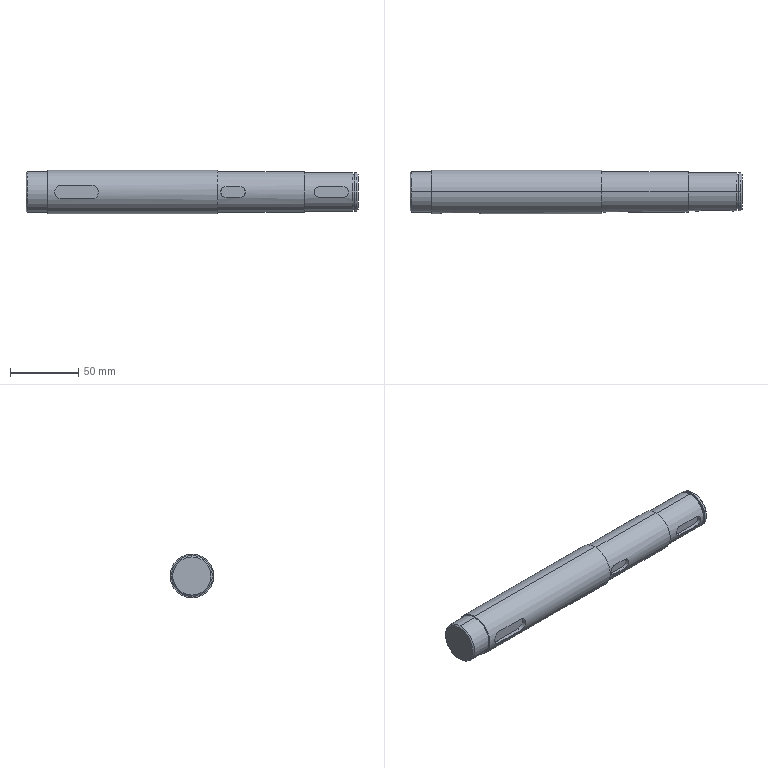Part | SolidWorks | features BaseBody 1 | 1 solid | 38 faces | box 243 x 32 x 32 mm | volume 178150 mm3 | cylinder 18 | plane 16 | cone 4 | commonest cylinder face diameters 8 x4 28 x4 30 x4 10 x2 25 x2 32 x2
STEP:
#1=CARTESIAN_POINT('',(16.,0.,-16.));
#2=VERTEX_POINT('',#1);
#3=CARTESIAN_POINT('',(16.,0.,16.));
#4=VERTEX_POINT('',#3);
#5=CARTESIAN_POINT('',(16.,0.,0.));
#6=DIRECTION('',(1.,0.,0.));
#7=DIRECTION('',(0.,0.,-1.));
#8=AXIS2_PLACEMENT_3D('',#5,#6,#7);
#9=CIRCLE('',#8,16.);
#10=EDGE_CURVE('',#2,#4,#9,.T.);
#11=ORIENTED_EDGE('',*,*,#10,.T.);
#12=CARTESIAN_POINT('',(140.5,0.,16.));
#13=VERTEX_POINT('',#12);
#14=CARTESIAN_POINT('',(78.25,0.,16.));
#15=DIRECTION('',(1.,0.,0.));
#16=VECTOR('',#15,1000.);
#17=LINE('',#14,#16);
#18=EDGE_CURVE('',#4,#13,#17,.T.);
#19=ORIENTED_EDGE('',*,*,#18,.T.);
#20=CARTESIAN_POINT('',(140.5,0.,-16.));
#21=VERTEX_POINT('',#20);
#22=CARTESIAN_POINT('',(140.5,0.,0.));
#23=DIRECTION('',(-1.,0.,0.));
#24=DIRECTION('',(0.,0.,-1.));
#25=AXIS2_PLACEMENT_3D('',#22,#23,#24);
#26=CIRCLE('',#25,16.);
#27=EDGE_CURVE('',#13,#21,#26,.T.);
#28=ORIENTED_EDGE('',*,*,#27,.T.);
#29=CARTESIAN_POINT('',(78.25,0.,-16.));
#30=DIRECTION('',(1.,0.,0.));
#31=VECTOR('',#30,1000.);
#32=LINE('',#29,#31);
#33=EDGE_CURVE('',#2,#21,#32,.T.);
#34=ORIENTED_EDGE('',*,*,#33,.F.);
#35=EDGE_LOOP('',(#11,#19,#28,#34));
#36=FACE_OUTER_BOUND('',#35,.T.);
#37=CARTESIAN_POINT('',(78.25,0.,0.));
#38=DIRECTION('',(1.,0.,0.));
#39=DIRECTION('',(0.,0.,-1.));
#40=AXIS2_PLACEMENT_3D('',#37,#38,#39);
#41=CYLINDRICAL_SURFACE('',#40,16.);
#42=ADVANCED_FACE('',(#36),#41,.T.);
#43=CARTESIAN_POINT('',(1.,0.,-15.));
#44=VERTEX_POINT('',#43);
#45=CARTESIAN_POINT('',(1.,0.,15.));
#46=VERTEX_POINT('',#45);
#47=CARTESIAN_POINT('',(1.,0.,0.));
#48=DIRECTION('',(1.,0.,0.));
#49=DIRECTION('',(0.,0.,-1.));
#50=AXIS2_PLACEMENT_3D('',#47,#48,#49);
#51=CIRCLE('',#50,15.);
#52=EDGE_CURVE('',#44,#46,#51,.T.);
#53=ORIENTED_EDGE('',*,*,#52,.T.);
#54=CARTESIAN_POINT('',(16.,0.,15.));
#55=VERTEX_POINT('',#54);
#56=CARTESIAN_POINT('',(8.,0.,15.));
#57=DIRECTION('',(1.,0.,0.));
#58=VECTOR('',#57,1000.);
#59=LINE('',#56,#58);
#60=EDGE_CURVE('',#46,#55,#59,.T.);
#61=ORIENTED_EDGE('',*,*,#60,.T.);
#62=CARTESIAN_POINT('',(16.,0.,-15.));
#63=VERTEX_POINT('',#62);
#64=CARTESIAN_POINT('',(16.,0.,0.));
#65=DIRECTION('',(1.,0.,0.));
#66=DIRECTION('',(0.,0.,-1.));
#67=AXIS2_PLACEMENT_3D('',#64,#65,#66);
#68=CIRCLE('',#67,15.);
#69=EDGE_CURVE('',#63,#55,#68,.T.);
#70=ORIENTED_EDGE('',*,*,#69,.F.);
#71=CARTESIAN_POINT('',(8.,0.,-15.));
#72=DIRECTION('',(1.,0.,0.));
#73=VECTOR('',#72,1000.);
#74=LINE('',#71,#73);
#75=EDGE_CURVE('',#44,#63,#74,.T.);
#76=ORIENTED_EDGE('',*,*,#75,.F.);
#77=EDGE_LOOP('',(#53,#61,#70,#76));
#78=FACE_OUTER_BOUND('',#77,.T.);
#79=CARTESIAN_POINT('',(8.,0.,0.));
#80=DIRECTION('',(1.,0.,0.));
#81=DIRECTION('',(0.,0.,-1.));
#82=AXIS2_PLACEMENT_3D('',#79,#80,#81);
#83=CYLINDRICAL_SURFACE('',#82,15.);
#84=ADVANCED_FACE('',(#78),#83,.T.);
#85=CARTESIAN_POINT('',(140.5,0.,15.));
#86=VERTEX_POINT('',#85);
#87=CARTESIAN_POINT('',(140.5,0.,-15.));
#88=VERTEX_POINT('',#87);
#89=CARTESIAN_POINT('',(140.5,0.,0.));
#90=DIRECTION('',(-1.,0.,0.));
#91=DIRECTION('',(0.,0.,-1.));
#92=AXIS2_PLACEMENT_3D('',#89,#90,#91);
#93=CIRCLE('',#92,15.);
#94=EDGE_CURVE('',#86,#88,#93,.T.);
#95=ORIENTED_EDGE('',*,*,#94,.F.);
#96=CARTESIAN_POINT('',(203.5,0.,15.));
#97=VERTEX_POINT('',#96);
#98=CARTESIAN_POINT('',(172.,0.,15.));
#99=DIRECTION('',(1.,0.,0.));
#100=VECTOR('',#99,1000.);
#101=LINE('',#98,#100);
#102=EDGE_CURVE('',#86,#97,#101,.T.);
#103=ORIENTED_EDGE('',*,*,#102,.T.);
#104=CARTESIAN_POINT('',(203.5,0.,-15.));
#105=VERTEX_POINT('',#104);
#106=CARTESIAN_POINT('',(203.5,0.,0.));
#107=DIRECTION('',(-1.,0.,0.));
#108=DIRECTION('',(0.,0.,-1.));
#109=AXIS2_PLACEMENT_3D('',#106,#107,#108);
#110=CIRCLE('',#109,15.);
#111=EDGE_CURVE('',#97,#105,#110,.T.);
#112=ORIENTED_EDGE('',*,*,#111,.T.);
#113=CARTESIAN_POINT('',(172.,0.,-15.));
#114=DIRECTION('',(1.,0.,0.));
#115=VECTOR('',#114,1000.);
#116=LINE('',#113,#115);
#117=EDGE_CURVE('',#88,#105,#116,.T.);
#118=ORIENTED_EDGE('',*,*,#117,.F.);
#119=EDGE_LOOP('',(#95,#103,#112,#118));
#120=FACE_OUTER_BOUND('',#119,.T.);
#121=CARTESIAN_POINT('',(172.,0.,0.));
#122=DIRECTION('',(1.,0.,0.));
#123=DIRECTION('',(0.,0.,-1.));
#124=AXIS2_PLACEMENT_3D('',#121,#122,#123);
#125=CYLINDRICAL_SURFACE('',#124,15.);
#126=ADVANCED_FACE('',(#120),#125,.T.);
#127=CARTESIAN_POINT('',(0.,0.,-14.));
#128=VERTEX_POINT('',#127);
#129=CARTESIAN_POINT('',(0.,0.,14.));
#130=VERTEX_POINT('',#129);
#131=CARTESIAN_POINT('',(0.,0.,0.));
#132=DIRECTION('',(1.,0.,0.));
#133=DIRECTION('',(0.,0.,-1.));
#134=AXIS2_PLACEMENT_3D('',#131,#132,#133);
#135=CIRCLE('',#134,14.);
#136=EDGE_CURVE('',#128,#130,#135,.T.);
#137=ORIENTED_EDGE('',*,*,#136,.T.);
#138=CARTESIAN_POINT('',(1.,0.,15.));
#139=DIRECTION('',(0.7071,0.,0.7071));
#140=VECTOR('',#139,1000.);
#141=LINE('',#138,#140);
#142=EDGE_CURVE('',#130,#46,#141,.T.);
#143=ORIENTED_EDGE('',*,*,#142,.T.);
#144=ORIENTED_EDGE('',*,*,#52,.F.);
#145=CARTESIAN_POINT('',(1.,0.,-15.));
#146=DIRECTION('',(0.7071,0.,-0.7071));
#147=VECTOR('',#146,1000.);
#148=LINE('',#145,#147);
#149=EDGE_CURVE('',#128,#44,#148,.T.);
#150=ORIENTED_EDGE('',*,*,#149,.F.);
#151=EDGE_LOOP('',(#137,#143,#144,#150));
#152=FACE_OUTER_BOUND('',#151,.T.);
#153=CARTESIAN_POINT('',(1.,0.,0.));
#154=DIRECTION('',(1.,0.,0.));
#155=DIRECTION('',(0.,0.,-1.));
#156=AXIS2_PLACEMENT_3D('',#153,#154,#155);
#157=CONICAL_SURFACE('',#156,15.,0.7854);
#158=ADVANCED_FACE('',(#152),#157,.T.);
#159=CARTESIAN_POINT('',(203.5,0.,14.));
#160=VERTEX_POINT('',#159);
#161=CARTESIAN_POINT('',(203.5,0.,-14.));
#162=VERTEX_POINT('',#161);
#163=CARTESIAN_POINT('',(203.5,0.,0.));
#164=DIRECTION('',(-1.,0.,0.));
#165=DIRECTION('',(0.,0.,-1.));
#166=AXIS2_PLACEMENT_3D('',#163,#164,#165);
#167=CIRCLE('',#166,14.);
#168=EDGE_CURVE('',#160,#162,#167,.T.);
#169=ORIENTED_EDGE('',*,*,#168,.F.);
#170=CARTESIAN_POINT('',(239.,0.,14.));
#171=VERTEX_POINT('',#170);
#172=CARTESIAN_POINT('',(221.25,0.,14.));
#173=DIRECTION('',(1.,0.,0.));
#174=VECTOR('',#173,1000.);
#175=LINE('',#172,#174);
#176=EDGE_CURVE('',#160,#171,#175,.T.);
#177=ORIENTED_EDGE('',*,*,#176,.T.);
#178=CARTESIAN_POINT('',(239.,0.,-14.));
#179=VERTEX_POINT('',#178);
#180=CARTESIAN_POINT('',(239.,0.,0.));
#181=DIRECTION('',(-1.,0.,0.));
#182=DIRECTION('',(0.,0.,-1.));
#183=AXIS2_PLACEMENT_3D('',#180,#181,#182);
#184=CIRCLE('',#183,14.);
#185=EDGE_CURVE('',#171,#179,#184,.T.);
#186=ORIENTED_EDGE('',*,*,#185,.T.);
#187=CARTESIAN_POINT('',(221.25,0.,-14.));
#188=DIRECTION('',(1.,0.,0.));
#189=VECTOR('',#188,1000.);
#190=LINE('',#187,#189);
#191=EDGE_CURVE('',#162,#179,#190,.T.);
#192=ORIENTED_EDGE('',*,*,#191,.F.);
#193=EDGE_LOOP('',(#169,#177,#186,#192));
#194=FACE_OUTER_BOUND('',#193,.T.);
#195=CARTESIAN_POINT('',(221.25,0.,0.));
#196=DIRECTION('',(1.,0.,0.));
#197=DIRECTION('',(0.,0.,-1.));
#198=AXIS2_PLACEMENT_3D('',#195,#196,#197);
#199=CYLINDRICAL_SURFACE('',#198,14.);
#200=ADVANCED_FACE('',(#194),#199,.T.);
#201=CARTESIAN_POINT('',(239.,0.,12.5));
#202=VERTEX_POINT('',#201);
#203=CARTESIAN_POINT('',(239.,0.,-12.5));
#204=VERTEX_POINT('',#203);
#205=CARTESIAN_POINT('',(239.,0.,0.));
#206=DIRECTION('',(-1.,0.,0.));
#207=DIRECTION('',(0.,0.,-1.));
#208=AXIS2_PLACEMENT_3D('',#205,#206,#207);
#209=CIRCLE('',#208,12.5);
#210=EDGE_CURVE('',#202,#204,#209,.T.);
#211=ORIENTED_EDGE('',*,*,#210,.F.);
#212=CARTESIAN_POINT('',(240.5,0.,12.5));
#213=VERTEX_POINT('',#212);
#214=CARTESIAN_POINT('',(239.75,0.,12.5));
#215=DIRECTION('',(1.,0.,0.));
#216=VECTOR('',#215,1000.);
#217=LINE('',#214,#216);
#218=EDGE_CURVE('',#202,#213,#217,.T.);
#219=ORIENTED_EDGE('',*,*,#218,.T.);
#220=CARTESIAN_POINT('',(240.5,0.,-12.5));
#221=VERTEX_POINT('',#220);
#222=CARTESIAN_POINT('',(240.5,0.,0.));
#223=DIRECTION('',(-1.,0.,0.));
#224=DIRECTION('',(0.,0.,-1.));
#225=AXIS2_PLACEMENT_3D('',#222,#223,#224);
#226=CIRCLE('',#225,12.5);
#227=EDGE_CURVE('',#213,#221,#226,.T.);
#228=ORIENTED_EDGE('',*,*,#227,.T.);
#229=CARTESIAN_POINT('',(239.75,0.,-12.5));
#230=DIRECTION('',(1.,0.,0.));
#231=VECTOR('',#230,1000.);
#232=LINE('',#229,#231);
#233=EDGE_CURVE('',#204,#221,#232,.T.);
#234=ORIENTED_EDGE('',*,*,#233,.F.);
#235=EDGE_LOOP('',(#211,#219,#228,#234));
#236=FACE_OUTER_BOUND('',#235,.T.);
#237=CARTESIAN_POINT('',(239.75,0.,0.));
#238=DIRECTION('',(1.,0.,0.));
#239=DIRECTION('',(0.,0.,-1.));
#240=AXIS2_PLACEMENT_3D('',#237,#238,#239);
#241=CYLINDRICAL_SURFACE('',#240,12.5);
#242=ADVANCED_FACE('',(#236),#241,.T.);
#243=CARTESIAN_POINT('',(240.5,0.,14.));
#244=VERTEX_POINT('',#243);
#245=CARTESIAN_POINT('',(240.5,0.,-14.));
#246=VERTEX_POINT('',#245);
#247=CARTESIAN_POINT('',(240.5,0.,0.));
#248=DIRECTION('',(-1.,0.,0.));
#249=DIRECTION('',(0.,0.,-1.));
#250=AXIS2_PLACEMENT_3D('',#247,#248,#249);
#251=CIRCLE('',#250,14.);
#252=EDGE_CURVE('',#244,#246,#251,.T.);
#253=ORIENTED_EDGE('',*,*,#252,.F.);
#254=CARTESIAN_POINT('',(242.,0.,14.));
#255=VERTEX_POINT('',#254);
#256=CARTESIAN_POINT('',(241.75,0.,14.));
#257=DIRECTION('',(1.,0.,0.));
#258=VECTOR('',#257,1000.);
#259=LINE('',#256,#258);
#260=EDGE_CURVE('',#244,#255,#259,.T.);
#261=ORIENTED_EDGE('',*,*,#260,.T.);
#262=CARTESIAN_POINT('',(242.,0.,-14.));
#263=VERTEX_POINT('',#262);
#264=CARTESIAN_POINT('',(242.,0.,0.));
#265=DIRECTION('',(-1.,0.,0.));
#266=DIRECTION('',(0.,0.,-1.));
#267=AXIS2_PLACEMENT_3D('',#264,#265,#266);
#268=CIRCLE('',#267,14.);
#269=EDGE_CURVE('',#255,#263,#268,.T.);
#270=ORIENTED_EDGE('',*,*,#269,.T.);
#271=CARTESIAN_POINT('',(241.75,0.,-14.));
#272=DIRECTION('',(1.,0.,0.));
#273=VECTOR('',#272,1000.);
#274=LINE('',#271,#273);
#275=EDGE_CURVE('',#246,#263,#274,.T.);
#276=ORIENTED_EDGE('',*,*,#275,.F.);
#277=EDGE_LOOP('',(#253,#261,#270,#276));
#278=FACE_OUTER_BOUND('',#277,.T.);
#279=CARTESIAN_POINT('',(241.75,0.,0.));
#280=DIRECTION('',(1.,0.,0.));
#281=DIRECTION('',(0.,0.,-1.));
#282=AXIS2_PLACEMENT_3D('',#279,#280,#281);
#283=CYLINDRICAL_SURFACE('',#282,14.);
#284=ADVANCED_FACE('',(#278),#283,.T.);
#285=CARTESIAN_POINT('',(243.,0.,13.));
#286=VERTEX_POINT('',#285);
#287=CARTESIAN_POINT('',(243.,0.,-13.));
#288=VERTEX_POINT('',#287);
#289=CARTESIAN_POINT('',(243.,0.,0.));
#290=DIRECTION('',(-1.,0.,0.));
#291=DIRECTION('',(0.,0.,1.));
#292=AXIS2_PLACEMENT_3D('',#289,#290,#291);
#293=CIRCLE('',#292,13.);
#294=EDGE_CURVE('',#286,#288,#293,.T.);
#295=ORIENTED_EDGE('',*,*,#294,.T.);
#296=CARTESIAN_POINT('',(242.,0.,-14.));
#297=DIRECTION('',(-0.7071,0.,-0.7071));
#298=VECTOR('',#297,1000.);
#299=LINE('',#296,#298);
#300=EDGE_CURVE('',#288,#263,#299,.T.);
#301=ORIENTED_EDGE('',*,*,#300,.T.);
#302=ORIENTED_EDGE('',*,*,#269,.F.);
#303=CARTESIAN_POINT('',(242.,0.,14.));
#304=DIRECTION('',(-0.7071,0.,0.7071));
#305=VECTOR('',#304,1000.);
#306=LINE('',#303,#305);
#307=EDGE_CURVE('',#286,#255,#306,.T.);
#308=ORIENTED_EDGE('',*,*,#307,.F.);
#309=EDGE_LOOP('',(#295,#301,#302,#308));
#310=FACE_OUTER_BOUND('',#309,.T.);
#311=CARTESIAN_POINT('',(242.,0.,0.));
#312=DIRECTION('',(-1.,0.,0.));
#313=DIRECTION('',(0.,0.,1.));
#314=AXIS2_PLACEMENT_3D('',#311,#312,#313);
#315=CONICAL_SURFACE('',#314,14.,0.7854);
#316=ADVANCED_FACE('',(#310),#315,.T.);
#317=ORIENTED_EDGE('',*,*,#18,.F.);
#318=CARTESIAN_POINT('',(16.,0.,0.));
#319=DIRECTION('',(1.,0.,0.));
#320=DIRECTION('',(0.,0.,-1.));
#321=AXIS2_PLACEMENT_3D('',#318,#319,#320);
#322=CIRCLE('',#321,16.);
#323=EDGE_CURVE('',#4,#2,#322,.T.);
#324=ORIENTED_EDGE('',*,*,#323,.T.);
#325=ORIENTED_EDGE('',*,*,#33,.T.);
#326=CARTESIAN_POINT('',(140.5,0.,0.));
#327=DIRECTION('',(-1.,0.,0.));
#328=DIRECTION('',(0.,0.,-1.));
#329=AXIS2_PLACEMENT_3D('',#326,#327,#328);
#330=CIRCLE('',#329,16.);
#331=EDGE_CURVE('',#21,#13,#330,.T.);
#332=ORIENTED_EDGE('',*,*,#331,.T.);
#333=EDGE_LOOP('',(#317,#324,#325,#332));
#334=FACE_OUTER_BOUND('',#333,.T.);
#335=CARTESIAN_POINT('',(26.,-15.199,5.));
#336=VERTEX_POINT('',#335);
#337=CARTESIAN_POINT('',(48.,-15.199,5.));
#338=VERTEX_POINT('',#337);
#339=CARTESIAN_POINT('',(78.25,-15.199,5.));
#340=DIRECTION('',(1.,0.,0.));
#341=VECTOR('',#340,1000.);
#342=LINE('',#339,#341);
#343=EDGE_CURVE('',#336,#338,#342,.T.);
#344=ORIENTED_EDGE('',*,*,#343,.T.);
#345=CARTESIAN_POINT('',(48.,-15.199,-5.));
#346=VERTEX_POINT('',#345);
#347=CARTESIAN_POINT('',(48.,-15.199,5.));
#348=CARTESIAN_POINT('',(48.332,-15.199,5.));
#349=CARTESIAN_POINT('',(48.659,-15.21,4.967));
#350=CARTESIAN_POINT('',(49.3,-15.251,4.839));
#351=CARTESIAN_POINT('',(49.619,-15.282,4.742));
#352=CARTESIAN_POINT('',(50.223,-15.357,4.491));
#353=CARTESIAN_POINT('',(50.509,-15.402,4.337));
#354=CARTESIAN_POINT('',(51.051,-15.5,3.975));
#355=CARTESIAN_POINT('',(51.305,-15.552,3.765));
#356=CARTESIAN_POINT('',(51.763,-15.656,3.308));
#357=CARTESIAN_POINT('',(51.97,-15.708,3.058));
#358=CARTESIAN_POINT('',(52.335,-15.804,2.512));
#359=CARTESIAN_POINT('',(52.49,-15.847,2.225));
#360=CARTESIAN_POINT('',(52.74,-15.92,1.624));
#361=CARTESIAN_POINT('',(52.837,-15.95,1.308));
#362=CARTESIAN_POINT('',(52.967,-15.99,0.6603));
#363=CARTESIAN_POINT('',(53.,-16.,0.3323));
#364=CARTESIAN_POINT('',(53.,-16.,-0.3324));
#365=CARTESIAN_POINT('',(52.967,-15.99,-0.6589));
#366=CARTESIAN_POINT('',(52.839,-15.95,-1.3));
#367=CARTESIAN_POINT('',(52.742,-15.921,-1.619));
#368=CARTESIAN_POINT('',(52.49,-15.848,-2.223));
#369=CARTESIAN_POINT('',(52.337,-15.804,-2.51));
#370=CARTESIAN_POINT('',(51.974,-15.709,-3.051));
#371=CARTESIAN_POINT('',(51.765,-15.656,-3.306));
#372=CARTESIAN_POINT('',(51.307,-15.553,-3.764));
#373=CARTESIAN_POINT('',(51.057,-15.501,-3.97));
#374=CARTESIAN_POINT('',(50.512,-15.402,-4.336));
#375=CARTESIAN_POINT('',(50.224,-15.358,-4.49));
#376=CARTESIAN_POINT('',(49.624,-15.282,-4.74));
#377=CARTESIAN_POINT('',(49.308,-15.251,-4.837));
#378=CARTESIAN_POINT('',(48.66,-15.21,-4.967));
#379=CARTESIAN_POINT('',(48.332,-15.199,-5.));
#380=CARTESIAN_POINT('',(48.,-15.199,-5.));
#381=B_SPLINE_CURVE_WITH_KNOTS('',3,(#347,#348,#349,#350,#351,#352,#353,#354,#355,#356,#357,#358,#359,#360,#361,#362,#363,#364,#365,#366,#367,#368,#369,#370,#371,#372,#373,#374,#375,#376,#377,#378,#379,#380),.UNSPECIFIED.,.F.,.F.,(4,2,2,2,2,2,2,2,2,2,2,2,2,2,2,2,4),(-0.00786,-0.006878,-0.005895,-0.004913,-0.00393,-0.002948,-0.001965,-0.0009825,0.000000059,0.0009826,0.001965,0.002948,0.00393,0.004913,0.005895,0.006878,0.007861),.UNSPECIFIED.);
#382=EDGE_CURVE('',#338,#346,#381,.T.);
#383=ORIENTED_EDGE('',*,*,#382,.T.);
#384=CARTESIAN_POINT('',(26.,-15.199,-5.));
#385=VERTEX_POINT('',#384);
#386=CARTESIAN_POINT('',(78.25,-15.199,-5.));
#387=DIRECTION('',(-1.,0.,0.));
#388=VECTOR('',#387,1000.);
#389=LINE('',#386,#388);
#390=EDGE_CURVE('',#346,#385,#389,.T.);
#391=ORIENTED_EDGE('',*,*,#390,.T.);
#392=CARTESIAN_POINT('',(26.,-15.199,-5.));
#393=CARTESIAN_POINT('',(25.668,-15.199,-5.));
#394=CARTESIAN_POINT('',(25.341,-15.21,-4.967));
#395=CARTESIAN_POINT('',(24.7,-15.251,-4.839));
#396=CARTESIAN_POINT('',(24.381,-15.282,-4.742));
#397=CARTESIAN_POINT('',(23.777,-15.357,-4.491));
#398=CARTESIAN_POINT('',(23.491,-15.402,-4.337));
#399=CARTESIAN_POINT('',(22.949,-15.5,-3.975));
#400=CARTESIAN_POINT('',(22.695,-15.552,-3.765));
#401=CARTESIAN_POINT('',(22.237,-15.656,-3.308));
#402=CARTESIAN_POINT('',(22.03,-15.708,-3.058));
#403=CARTESIAN_POINT('',(21.665,-15.804,-2.512));
#404=CARTESIAN_POINT('',(21.51,-15.847,-2.225));
#405=CARTESIAN_POINT('',(21.26,-15.92,-1.624));
#406=CARTESIAN_POINT('',(21.163,-15.95,-1.308));
#407=CARTESIAN_POINT('',(21.033,-15.99,-0.6603));
#408=CARTESIAN_POINT('',(21.,-16.,-0.3323));
#409=CARTESIAN_POINT('',(21.,-16.,0.3324));
#410=CARTESIAN_POINT('',(21.033,-15.99,0.6589));
#411=CARTESIAN_POINT('',(21.161,-15.95,1.3));
#412=CARTESIAN_POINT('',(21.258,-15.921,1.619));
#413=CARTESIAN_POINT('',(21.51,-15.848,2.223));
#414=CARTESIAN_POINT('',(21.663,-15.804,2.51));
#415=CARTESIAN_POINT('',(22.026,-15.709,3.051));
#416=CARTESIAN_POINT('',(22.235,-15.656,3.306));
#417=CARTESIAN_POINT('',(22.693,-15.553,3.764));
#418=CARTESIAN_POINT('',(22.943,-15.501,3.97));
#419=CARTESIAN_POINT('',(23.488,-15.402,4.336));
#420=CARTESIAN_POINT('',(23.776,-15.358,4.49));
#421=CARTESIAN_POINT('',(24.376,-15.282,4.74));
#422=CARTESIAN_POINT('',(24.692,-15.251,4.837));
#423=CARTESIAN_POINT('',(25.34,-15.21,4.967));
#424=CARTESIAN_POINT('',(25.668,-15.199,5.));
#425=CARTESIAN_POINT('',(26.,-15.199,5.));
#426=B_SPLINE_CURVE_WITH_KNOTS('',3,(#392,#393,#394,#395,#396,#397,#398,#399,#400,#401,#402,#403,#404,#405,#406,#407,#408,#409,#410,#411,#412,#413,#414,#415,#416,#417,#418,#419,#420,#421,#422,#423,#424,#425),.UNSPECIFIED.,.F.,.F.,(4,2,2,2,2,2,2,2,2,2,2,2,2,2,2,2,4),(0.,0.0009826,0.001965,0.002948,0.00393,0.004913,0.005895,0.006878,0.00786,0.008843,0.009826,0.01081,0.01179,0.01277,0.01376,0.01474,0.01572),.UNSPECIFIED.);
#427=EDGE_CURVE('',#385,#336,#426,.T.);
#428=ORIENTED_EDGE('',*,*,#427,.T.);
#429=EDGE_LOOP('',(#344,#383,#391,#428));
#430=FACE_BOUND('',#429,.T.);
#431=CARTESIAN_POINT('',(78.25,0.,0.));
#432=DIRECTION('',(1.,0.,0.));
#433=DIRECTION('',(0.,0.,-1.));
#434=AXIS2_PLACEMENT_3D('',#431,#432,#433);
#435=CYLINDRICAL_SURFACE('',#434,16.);
#436=ADVANCED_FACE('',(#334,#430),#435,.T.);
#437=ORIENTED_EDGE('',*,*,#69,.T.);
#438=CARTESIAN_POINT('',(16.,0.,0.));
#439=DIRECTION('',(1.,0.,0.));
#440=DIRECTION('',(0.,0.,-1.));
#441=AXIS2_PLACEMENT_3D('',#438,#439,#440);
#442=CIRCLE('',#441,15.);
#443=EDGE_CURVE('',#55,#63,#442,.T.);
#444=ORIENTED_EDGE('',*,*,#443,.T.);
#445=EDGE_LOOP('',(#437,#444));
#446=FACE_BOUND('',#445,.T.);
#447=ORIENTED_EDGE('',*,*,#10,.F.);
#448=ORIENTED_EDGE('',*,*,#323,.F.);
#449=EDGE_LOOP('',(#447,#448));
#450=FACE_OUTER_BOUND('',#449,.T.);
#451=CARTESIAN_POINT('',(16.,15.5,0.));
#452=DIRECTION('',(-1.,0.,0.));
#453=DIRECTION('',(0.,0.,1.));
#454=AXIS2_PLACEMENT_3D('',#451,#452,#453);
#455=PLANE('',#454);
#456=ADVANCED_FACE('',(#446,#450),#455,.T.);
#457=ORIENTED_EDGE('',*,*,#382,.F.);
#458=CARTESIAN_POINT('',(48.,-12.5,5.));
#459=VERTEX_POINT('',#458);
#460=CARTESIAN_POINT('',(48.,-12.5,5.));
#461=DIRECTION('',(0.,-1.,0.));
#462=VECTOR('',#461,1000.);
#463=LINE('',#460,#462);
#464=EDGE_CURVE('',#459,#338,#463,.T.);
#465=ORIENTED_EDGE('',*,*,#464,.F.);
#466=CARTESIAN_POINT('',(48.,-12.5,-5.));
#467=VERTEX_POINT('',#466);
#468=CARTESIAN_POINT('',(48.,-12.5,0.));
#469=DIRECTION('',(0.,-1.,0.));
#470=DIRECTION('',(0.,0.,-1.));
#471=AXIS2_PLACEMENT_3D('',#468,#469,#470);
#472=CIRCLE('',#471,5.);
#473=EDGE_CURVE('',#467,#459,#472,.T.);
#474=ORIENTED_EDGE('',*,*,#473,.F.);
#475=CARTESIAN_POINT('',(48.,-12.5,-5.));
#476=DIRECTION('',(0.,1.,0.));
#477=VECTOR('',#476,1000.);
#478=LINE('',#475,#477);
#479=EDGE_CURVE('',#346,#467,#478,.T.);
#480=ORIENTED_EDGE('',*,*,#479,.F.);
#481=EDGE_LOOP('',(#457,#465,#474,#480));
#482=FACE_OUTER_BOUND('',#481,.T.);
#483=CARTESIAN_POINT('',(48.,-12.5,0.));
#484=DIRECTION('',(0.,-1.,0.));
#485=DIRECTION('',(0.,0.,-1.));
#486=AXIS2_PLACEMENT_3D('',#483,#484,#485);
#487=CYLINDRICAL_SURFACE('',#486,5.);
#488=ADVANCED_FACE('',(#482),#487,.F.);
#489=CARTESIAN_POINT('',(26.,-12.5,5.));
#490=VERTEX_POINT('',#489);
#491=CARTESIAN_POINT('',(26.,-16.,5.));
#492=DIRECTION('',(0.,-1.,0.));
#493=VECTOR('',#492,1000.);
#494=LINE('',#491,#493);
#495=EDGE_CURVE('',#490,#336,#494,.T.);
#496=ORIENTED_EDGE('',*,*,#495,.F.);
#497=CARTESIAN_POINT('',(26.,-12.5,5.));
#498=DIRECTION('',(-1.,0.,0.));
#499=VECTOR('',#498,1000.);
#500=LINE('',#497,#499);
#501=EDGE_CURVE('',#459,#490,#500,.T.);
#502=ORIENTED_EDGE('',*,*,#501,.F.);
#503=ORIENTED_EDGE('',*,*,#464,.T.);
#504=ORIENTED_EDGE('',*,*,#343,.F.);
#505=EDGE_LOOP('',(#496,#502,#503,#504));
#506=FACE_OUTER_BOUND('',#505,.T.);
#507=CARTESIAN_POINT('',(26.,-16.,5.));
#508=DIRECTION('',(0.,0.,1.));
#509=DIRECTION('',(0.,-1.,0.));
#510=AXIS2_PLACEMENT_3D('',#507,#508,#509);
#511=PLANE('',#510);
#512=ADVANCED_FACE('',(#506),#511,.F.);
#513=CARTESIAN_POINT('',(26.,-12.5,-5.));
#514=VERTEX_POINT('',#513);
#515=CARTESIAN_POINT('',(26.,-12.5,0.));
#516=DIRECTION('',(0.,-1.,0.));
#517=DIRECTION('',(0.,0.,-1.));
#518=AXIS2_PLACEMENT_3D('',#515,#516,#517);
#519=CIRCLE('',#518,5.);
#520=EDGE_CURVE('',#490,#514,#519,.T.);
#521=ORIENTED_EDGE('',*,*,#520,.F.);
#522=ORIENTED_EDGE('',*,*,#495,.T.);
#523=ORIENTED_EDGE('',*,*,#427,.F.);
#524=CARTESIAN_POINT('',(26.,-12.5,-5.));
#525=DIRECTION('',(0.,-1.,0.));
#526=VECTOR('',#525,1000.);
#527=LINE('',#524,#526);
#528=EDGE_CURVE('',#514,#385,#527,.T.);
#529=ORIENTED_EDGE('',*,*,#528,.F.);
#530=EDGE_LOOP('',(#521,#522,#523,#529));
#531=FACE_OUTER_BOUND('',#530,.T.);
#532=CARTESIAN_POINT('',(26.,-12.5,0.));
#533=DIRECTION('',(0.,-1.,0.));
#534=DIRECTION('',(0.,0.,-1.));
#535=AXIS2_PLACEMENT_3D('',#532,#533,#534);
#536=CYLINDRICAL_SURFACE('',#535,5.);
#537=ADVANCED_FACE('',(#531),#536,.F.);
#538=ORIENTED_EDGE('',*,*,#479,.T.);
#539=CARTESIAN_POINT('',(26.,-12.5,-5.));
#540=DIRECTION('',(1.,0.,0.));
#541=VECTOR('',#540,1000.);
#542=LINE('',#539,#541);
#543=EDGE_CURVE('',#514,#467,#542,.T.);
#544=ORIENTED_EDGE('',*,*,#543,.F.);
#545=ORIENTED_EDGE('',*,*,#528,.T.);
#546=ORIENTED_EDGE('',*,*,#390,.F.);
#547=EDGE_LOOP('',(#538,#544,#545,#546));
#548=FACE_OUTER_BOUND('',#547,.T.);
#549=CARTESIAN_POINT('',(26.,-12.5,-5.));
#550=DIRECTION('',(0.,0.,-1.));
#551=DIRECTION('',(0.,1.,0.));
#552=AXIS2_PLACEMENT_3D('',#549,#550,#551);
#553=PLANE('',#552);
#554=ADVANCED_FACE('',(#548),#553,.F.);
#555=CARTESIAN_POINT('',(140.5,0.,0.));
#556=DIRECTION('',(-1.,0.,0.));
#557=DIRECTION('',(0.,0.,-1.));
#558=AXIS2_PLACEMENT_3D('',#555,#556,#557);
#559=CIRCLE('',#558,15.);
#560=EDGE_CURVE('',#88,#86,#559,.T.);
#561=ORIENTED_EDGE('',*,*,#560,.T.);
#562=ORIENTED_EDGE('',*,*,#94,.T.);
#563=EDGE_LOOP('',(#561,#562));
#564=FACE_BOUND('',#563,.T.);
#565=ORIENTED_EDGE('',*,*,#331,.F.);
#566=ORIENTED_EDGE('',*,*,#27,.F.);
#567=EDGE_LOOP('',(#565,#566));
#568=FACE_OUTER_BOUND('',#567,.T.);
#569=CARTESIAN_POINT('',(140.5,15.5,0.));
#570=DIRECTION('',(1.,0.,0.));
#571=DIRECTION('',(0.,0.,-1.));
#572=AXIS2_PLACEMENT_3D('',#569,#570,#571);
#573=PLANE('',#572);
#574=ADVANCED_FACE('',(#564,#568),#573,.T.);
#575=ORIENTED_EDGE('',*,*,#60,.F.);
#576=CARTESIAN_POINT('',(1.,0.,0.));
#577=DIRECTION('',(1.,0.,0.));
#578=DIRECTION('',(0.,0.,-1.));
#579=AXIS2_PLACEMENT_3D('',#576,#577,#578);
#580=CIRCLE('',#579,15.);
#581=EDGE_CURVE('',#46,#44,#580,.T.);
#582=ORIENTED_EDGE('',*,*,#581,.T.);
#583=ORIENTED_EDGE('',*,*,#75,.T.);
#584=ORIENTED_EDGE('',*,*,#443,.F.);
#585=EDGE_LOOP('',(#575,#582,#583,#584));
#586=FACE_OUTER_BOUND('',#585,.T.);
#587=CARTESIAN_POINT('',(8.,0.,0.));
#588=DIRECTION('',(1.,0.,0.));
#589=DIRECTION('',(0.,0.,-1.));
#590=AXIS2_PLACEMENT_3D('',#587,#588,#589);
#591=CYLINDRICAL_SURFACE('',#590,15.);
#592=ADVANCED_FACE('',(#586),#591,.T.);
#593=ORIENTED_EDGE('',*,*,#520,.T.);
#594=ORIENTED_EDGE('',*,*,#543,.T.);
#595=ORIENTED_EDGE('',*,*,#473,.T.);
#596=ORIENTED_EDGE('',*,*,#501,.T.);
#597=EDGE_LOOP('',(#593,#594,#595,#596));
#598=FACE_OUTER_BOUND('',#597,.T.);
#599=CARTESIAN_POINT('',(26.,-12.5,5.));
#600=DIRECTION('',(0.,1.,0.));
#601=DIRECTION('',(0.,0.,1.));
#602=AXIS2_PLACEMENT_3D('',#599,#600,#601);
#603=PLANE('',#602);
#604=ADVANCED_FACE('',(#598),#603,.F.);
#605=ORIENTED_EDGE('',*,*,#102,.F.);
#606=ORIENTED_EDGE('',*,*,#560,.F.);
#607=ORIENTED_EDGE('',*,*,#117,.T.);
#608=CARTESIAN_POINT('',(203.5,0.,0.));
#609=DIRECTION('',(-1.,0.,0.));
#610=DIRECTION('',(0.,0.,-1.));
#611=AXIS2_PLACEMENT_3D('',#608,#609,#610);
#612=CIRCLE('',#611,15.);
#613=EDGE_CURVE('',#105,#97,#612,.T.);
#614=ORIENTED_EDGE('',*,*,#613,.T.);
#615=EDGE_LOOP('',(#605,#606,#607,#614));
#616=FACE_OUTER_BOUND('',#615,.T.);
#617=CARTESIAN_POINT('',(156.5,-14.457,-4.));
#618=VERTEX_POINT('',#617);
#619=CARTESIAN_POINT('',(146.5,-14.457,-4.));
#620=VERTEX_POINT('',#619);
#621=CARTESIAN_POINT('',(172.,-14.457,-4.));
#622=DIRECTION('',(-1.,0.,0.));
#623=VECTOR('',#622,1000.);
#624=LINE('',#621,#623);
#625=EDGE_CURVE('',#618,#620,#624,.T.);
#626=ORIENTED_EDGE('',*,*,#625,.T.);
#627=CARTESIAN_POINT('',(146.5,-14.457,4.));
#628=VERTEX_POINT('',#627);
#629=CARTESIAN_POINT('',(146.5,-14.457,-4.));
#630=CARTESIAN_POINT('',(146.235,-14.457,-4.));
#631=CARTESIAN_POINT('',(145.974,-14.464,-3.974));
#632=CARTESIAN_POINT('',(145.461,-14.492,-3.872));
#633=CARTESIAN_POINT('',(145.207,-14.513,-3.794));
#634=CARTESIAN_POINT('',(144.723,-14.564,-3.593));
#635=CARTESIAN_POINT('',(144.494,-14.594,-3.47));
#636=CARTESIAN_POINT('',(144.06,-14.66,-3.181));
#637=CARTESIAN_POINT('',(143.856,-14.696,-3.013));
#638=CARTESIAN_POINT('',(143.489,-14.766,-2.646));
#639=CARTESIAN_POINT('',(143.324,-14.801,-2.445));
#640=CARTESIAN_POINT('',(143.031,-14.866,-2.009));
#641=CARTESIAN_POINT('',(142.908,-14.896,-1.778));
#642=CARTESIAN_POINT('',(142.707,-14.946,-1.298));
#643=CARTESIAN_POINT('',(142.63,-14.966,-1.045));
#644=CARTESIAN_POINT('',(142.526,-14.993,-0.5274));
#645=CARTESIAN_POINT('',(142.5,-15.,-0.2653));
#646=CARTESIAN_POINT('',(142.5,-15.,0.2655));
#647=CARTESIAN_POINT('',(142.526,-14.993,0.5262));
#648=CARTESIAN_POINT('',(142.628,-14.966,1.039));
#649=CARTESIAN_POINT('',(142.706,-14.946,1.293));
#650=CARTESIAN_POINT('',(142.907,-14.896,1.777));
#651=CARTESIAN_POINT('',(143.03,-14.867,2.006));
#652=CARTESIAN_POINT('',(143.32,-14.802,2.44));
#653=CARTESIAN_POINT('',(143.488,-14.766,2.644));
#654=CARTESIAN_POINT('',(143.854,-14.696,3.011));
#655=CARTESIAN_POINT('',(144.055,-14.661,3.177));
#656=CARTESIAN_POINT('',(144.491,-14.594,3.469));
#657=CARTESIAN_POINT('',(144.722,-14.564,3.592));
#658=CARTESIAN_POINT('',(145.202,-14.513,3.793));
#659=CARTESIAN_POINT('',(145.455,-14.492,3.87));
#660=CARTESIAN_POINT('',(145.973,-14.464,3.974));
#661=CARTESIAN_POINT('',(146.235,-14.457,4.));
#662=CARTESIAN_POINT('',(146.5,-14.457,4.));
#663=B_SPLINE_CURVE_WITH_KNOTS('',3,(#629,#630,#631,#632,#633,#634,#635,#636,#637,#638,#639,#640,#641,#642,#643,#644,#645,#646,#647,#648,#649,#650,#651,#652,#653,#654,#655,#656,#657,#658,#659,#660,#661,#662),.UNSPECIFIED.,.F.,.F.,(4,2,2,2,2,2,2,2,2,2,2,2,2,2,2,2,4),(0.,0.0007847,0.001569,0.002354,0.003139,0.003923,0.004708,0.005493,0.006277,0.007062,0.007847,0.008631,0.009416,0.0102,0.01099,0.01177,0.01255),.UNSPECIFIED.);
#664=EDGE_CURVE('',#620,#628,#663,.T.);
#665=ORIENTED_EDGE('',*,*,#664,.T.);
#666=CARTESIAN_POINT('',(156.5,-14.457,4.));
#667=VERTEX_POINT('',#666);
#668=CARTESIAN_POINT('',(172.,-14.457,4.));
#669=DIRECTION('',(1.,0.,0.));
#670=VECTOR('',#669,1000.);
#671=LINE('',#668,#670);
#672=EDGE_CURVE('',#628,#667,#671,.T.);
#673=ORIENTED_EDGE('',*,*,#672,.T.);
#674=CARTESIAN_POINT('',(156.5,-14.457,4.));
#675=CARTESIAN_POINT('',(156.765,-14.457,4.));
#676=CARTESIAN_POINT('',(157.026,-14.464,3.974));
#677=CARTESIAN_POINT('',(157.539,-14.492,3.872));
#678=CARTESIAN_POINT('',(157.793,-14.513,3.794));
#679=CARTESIAN_POINT('',(158.277,-14.564,3.593));
#680=CARTESIAN_POINT('',(158.506,-14.594,3.47));
#681=CARTESIAN_POINT('',(158.94,-14.66,3.181));
#682=CARTESIAN_POINT('',(159.144,-14.696,3.013));
#683=CARTESIAN_POINT('',(159.511,-14.766,2.646));
#684=CARTESIAN_POINT('',(159.676,-14.801,2.445));
#685=CARTESIAN_POINT('',(159.969,-14.866,2.009));
#686=CARTESIAN_POINT('',(160.092,-14.896,1.778));
#687=CARTESIAN_POINT('',(160.293,-14.946,1.298));
#688=CARTESIAN_POINT('',(160.37,-14.966,1.045));
#689=CARTESIAN_POINT('',(160.474,-14.993,0.5274));
#690=CARTESIAN_POINT('',(160.5,-15.,0.2653));
#691=CARTESIAN_POINT('',(160.5,-15.,-0.2655));
#692=CARTESIAN_POINT('',(160.474,-14.993,-0.5262));
#693=CARTESIAN_POINT('',(160.372,-14.966,-1.039));
#694=CARTESIAN_POINT('',(160.294,-14.946,-1.293));
#695=CARTESIAN_POINT('',(160.093,-14.896,-1.777));
#696=CARTESIAN_POINT('',(159.97,-14.867,-2.006));
#697=CARTESIAN_POINT('',(159.68,-14.802,-2.44));
#698=CARTESIAN_POINT('',(159.512,-14.766,-2.644));
#699=CARTESIAN_POINT('',(159.146,-14.696,-3.011));
#700=CARTESIAN_POINT('',(158.945,-14.661,-3.177));
#701=CARTESIAN_POINT('',(158.509,-14.594,-3.469));
#702=CARTESIAN_POINT('',(158.278,-14.564,-3.592));
#703=CARTESIAN_POINT('',(157.798,-14.513,-3.793));
#704=CARTESIAN_POINT('',(157.545,-14.492,-3.87));
#705=CARTESIAN_POINT('',(157.027,-14.464,-3.974));
#706=CARTESIAN_POINT('',(156.765,-14.457,-4.));
#707=CARTESIAN_POINT('',(156.5,-14.457,-4.));
#708=B_SPLINE_CURVE_WITH_KNOTS('',3,(#674,#675,#676,#677,#678,#679,#680,#681,#682,#683,#684,#685,#686,#687,#688,#689,#690,#691,#692,#693,#694,#695,#696,#697,#698,#699,#700,#701,#702,#703,#704,#705,#706,#707),.UNSPECIFIED.,.F.,.F.,(4,2,2,2,2,2,2,2,2,2,2,2,2,2,2,2,4),(-0.006277,-0.005492,-0.004708,-0.003923,-0.003139,-0.002354,-0.001569,-0.0007846,0.000000075,0.0007847,0.001569,0.002354,0.003139,0.003923,0.004708,0.005493,0.006277),.UNSPECIFIED.);
#709=EDGE_CURVE('',#667,#618,#708,.T.);
#710=ORIENTED_EDGE('',*,*,#709,.T.);
#711=EDGE_LOOP('',(#626,#665,#673,#710));
#712=FACE_BOUND('',#711,.T.);
#713=CARTESIAN_POINT('',(172.,0.,0.));
#714=DIRECTION('',(1.,0.,0.));
#715=DIRECTION('',(0.,0.,-1.));
#716=AXIS2_PLACEMENT_3D('',#713,#714,#715);
#717=CYLINDRICAL_SURFACE('',#716,15.);
#718=ADVANCED_FACE('',(#616,#712),#717,.T.);
#719=ORIENTED_EDGE('',*,*,#142,.F.);
#720=CARTESIAN_POINT('',(0.,0.,0.));
#721=DIRECTION('',(1.,0.,0.));
#722=DIRECTION('',(0.,0.,-1.));
#723=AXIS2_PLACEMENT_3D('',#720,#721,#722);
#724=CIRCLE('',#723,14.);
#725=EDGE_CURVE('',#130,#128,#724,.T.);
#726=ORIENTED_EDGE('',*,*,#725,.T.);
#727=ORIENTED_EDGE('',*,*,#149,.T.);
#728=ORIENTED_EDGE('',*,*,#581,.F.);
#729=EDGE_LOOP('',(#719,#726,#727,#728));
#730=FACE_OUTER_BOUND('',#729,.T.);
#731=CARTESIAN_POINT('',(1.,0.,0.));
#732=DIRECTION('',(1.,0.,0.));
#733=DIRECTION('',(0.,0.,-1.));
#734=AXIS2_PLACEMENT_3D('',#731,#732,#733);
#735=CONICAL_SURFACE('',#734,15.,0.7854);
#736=ADVANCED_FACE('',(#730),#735,.T.);
#737=CARTESIAN_POINT('',(203.5,0.,0.));
#738=DIRECTION('',(-1.,0.,0.));
#739=DIRECTION('',(0.,0.,-1.));
#740=AXIS2_PLACEMENT_3D('',#737,#738,#739);
#741=CIRCLE('',#740,14.);
#742=EDGE_CURVE('',#162,#160,#741,.T.);
#743=ORIENTED_EDGE('',*,*,#742,.T.);
#744=ORIENTED_EDGE('',*,*,#168,.T.);
#745=EDGE_LOOP('',(#743,#744));
#746=FACE_BOUND('',#745,.T.);
#747=ORIENTED_EDGE('',*,*,#613,.F.);
#748=ORIENTED_EDGE('',*,*,#111,.F.);
#749=EDGE_LOOP('',(#747,#748));
#750=FACE_OUTER_BOUND('',#749,.T.);
#751=CARTESIAN_POINT('',(203.5,14.5,0.));
#752=DIRECTION('',(1.,0.,0.));
#753=DIRECTION('',(0.,0.,-1.));
#754=AXIS2_PLACEMENT_3D('',#751,#752,#753);
#755=PLANE('',#754);
#756=ADVANCED_FACE('',(#746,#750),#755,.T.);
#757=CARTESIAN_POINT('',(146.5,-12.,4.));
#758=VERTEX_POINT('',#757);
#759=CARTESIAN_POINT('',(146.5,-12.,4.));
#760=DIRECTION('',(0.,1.,0.));
#761=VECTOR('',#760,1000.);
#762=LINE('',#759,#761);
#763=EDGE_CURVE('',#628,#758,#762,.T.);
#764=ORIENTED_EDGE('',*,*,#763,.F.);
#765=ORIENTED_EDGE('',*,*,#664,.F.);
#766=CARTESIAN_POINT('',(146.5,-12.,-4.));
#767=VERTEX_POINT('',#766);
#768=CARTESIAN_POINT('',(146.5,-12.,-4.));
#769=DIRECTION('',(0.,-1.,0.));
#770=VECTOR('',#769,1000.);
#771=LINE('',#768,#770);
#772=EDGE_CURVE('',#767,#620,#771,.T.);
#773=ORIENTED_EDGE('',*,*,#772,.F.);
#774=CARTESIAN_POINT('',(146.5,-12.,0.));
#775=DIRECTION('',(0.,-1.,0.));
#776=DIRECTION('',(0.,0.,-1.));
#777=AXIS2_PLACEMENT_3D('',#774,#775,#776);
#778=CIRCLE('',#777,4.);
#779=EDGE_CURVE('',#758,#767,#778,.T.);
#780=ORIENTED_EDGE('',*,*,#779,.F.);
#781=EDGE_LOOP('',(#764,#765,#773,#780));
#782=FACE_OUTER_BOUND('',#781,.T.);
#783=CARTESIAN_POINT('',(146.5,-12.,0.));
#784=DIRECTION('',(0.,-1.,0.));
#785=DIRECTION('',(0.,0.,-1.));
#786=AXIS2_PLACEMENT_3D('',#783,#784,#785);
#787=CYLINDRICAL_SURFACE('',#786,4.);
#788=ADVANCED_FACE('',(#782),#787,.F.);
#789=CARTESIAN_POINT('',(156.5,-12.,-4.));
#790=VERTEX_POINT('',#789);
#791=CARTESIAN_POINT('',(156.5,-15.,-4.));
#792=DIRECTION('',(0.,-1.,0.));
#793=VECTOR('',#792,1000.);
#794=LINE('',#791,#793);
#795=EDGE_CURVE('',#790,#618,#794,.T.);
#796=ORIENTED_EDGE('',*,*,#795,.F.);
#797=CARTESIAN_POINT('',(156.5,-12.,-4.));
#798=DIRECTION('',(1.,0.,0.));
#799=VECTOR('',#798,1000.);
#800=LINE('',#797,#799);
#801=EDGE_CURVE('',#767,#790,#800,.T.);
#802=ORIENTED_EDGE('',*,*,#801,.F.);
#803=ORIENTED_EDGE('',*,*,#772,.T.);
#804=ORIENTED_EDGE('',*,*,#625,.F.);
#805=EDGE_LOOP('',(#796,#802,#803,#804));
#806=FACE_OUTER_BOUND('',#805,.T.);
#807=CARTESIAN_POINT('',(156.5,-15.,-4.));
#808=DIRECTION('',(0.,0.,-1.));
#809=DIRECTION('',(0.,1.,0.));
#810=AXIS2_PLACEMENT_3D('',#807,#808,#809);
#811=PLANE('',#810);
#812=ADVANCED_FACE('',(#806),#811,.F.);
#813=CARTESIAN_POINT('',(156.5,-12.,4.));
#814=VERTEX_POINT('',#813);
#815=CARTESIAN_POINT('',(156.5,-12.,0.));
#816=DIRECTION('',(0.,-1.,0.));
#817=DIRECTION('',(0.,0.,-1.));
#818=AXIS2_PLACEMENT_3D('',#815,#816,#817);
#819=CIRCLE('',#818,4.);
#820=EDGE_CURVE('',#790,#814,#819,.T.);
#821=ORIENTED_EDGE('',*,*,#820,.F.);
#822=ORIENTED_EDGE('',*,*,#795,.T.);
#823=ORIENTED_EDGE('',*,*,#709,.F.);
#824=CARTESIAN_POINT('',(156.5,-12.,4.));
#825=DIRECTION('',(0.,-1.,0.));
#826=VECTOR('',#825,1000.);
#827=LINE('',#824,#826);
#828=EDGE_CURVE('',#814,#667,#827,.T.);
#829=ORIENTED_EDGE('',*,*,#828,.F.);
#830=EDGE_LOOP('',(#821,#822,#823,#829));
#831=FACE_OUTER_BOUND('',#830,.T.);
#832=CARTESIAN_POINT('',(156.5,-12.,0.));
#833=DIRECTION('',(0.,-1.,0.));
#834=DIRECTION('',(0.,0.,-1.));
#835=AXIS2_PLACEMENT_3D('',#832,#833,#834);
#836=CYLINDRICAL_SURFACE('',#835,4.);
#837=ADVANCED_FACE('',(#831),#836,.F.);
#838=ORIENTED_EDGE('',*,*,#763,.T.);
#839=CARTESIAN_POINT('',(156.5,-12.,4.));
#840=DIRECTION('',(-1.,0.,0.));
#841=VECTOR('',#840,1000.);
#842=LINE('',#839,#841);
#843=EDGE_CURVE('',#814,#758,#842,.T.);
#844=ORIENTED_EDGE('',*,*,#843,.F.);
#845=ORIENTED_EDGE('',*,*,#828,.T.);
#846=ORIENTED_EDGE('',*,*,#672,.F.);
#847=EDGE_LOOP('',(#838,#844,#845,#846));
#848=FACE_OUTER_BOUND('',#847,.T.);
#849=CARTESIAN_POINT('',(156.5,-12.,4.));
#850=DIRECTION('',(0.,0.,1.));
#851=DIRECTION('',(0.,-1.,0.));
#852=AXIS2_PLACEMENT_3D('',#849,#850,#851);
#853=PLANE('',#852);
#854=ADVANCED_FACE('',(#848),#853,.F.);
#855=ORIENTED_EDGE('',*,*,#136,.F.);
#856=ORIENTED_EDGE('',*,*,#725,.F.);
#857=EDGE_LOOP('',(#855,#856));
#858=FACE_OUTER_BOUND('',#857,.T.);
#859=CARTESIAN_POINT('',(0.,7.5,0.));
#860=DIRECTION('',(-1.,0.,0.));
#861=DIRECTION('',(0.,0.,1.));
#862=AXIS2_PLACEMENT_3D('',#859,#860,#861);
#863=PLANE('',#862);
#864=ADVANCED_FACE('',(#858),#863,.T.);
#865=ORIENTED_EDGE('',*,*,#176,.F.);
#866=ORIENTED_EDGE('',*,*,#742,.F.);
#867=ORIENTED_EDGE('',*,*,#191,.T.);
#868=CARTESIAN_POINT('',(239.,0.,0.));
#869=DIRECTION('',(-1.,0.,0.));
#870=DIRECTION('',(0.,0.,-1.));
#871=AXIS2_PLACEMENT_3D('',#868,#869,#870);
#872=CIRCLE('',#871,14.);
#873=EDGE_CURVE('',#179,#171,#872,.T.);
#874=ORIENTED_EDGE('',*,*,#873,.T.);
#875=EDGE_LOOP('',(#865,#866,#867,#874));
#876=FACE_OUTER_BOUND('',#875,.T.);
#877=CARTESIAN_POINT('',(232.,-13.416,-4.));
#878=VERTEX_POINT('',#877);
#879=CARTESIAN_POINT('',(215.,-13.416,-4.));
#880=VERTEX_POINT('',#879);
#881=CARTESIAN_POINT('',(221.25,-13.416,-4.));
#882=DIRECTION('',(-1.,0.,0.));
#883=VECTOR('',#882,1000.);
#884=LINE('',#881,#883);
#885=EDGE_CURVE('',#878,#880,#884,.T.);
#886=ORIENTED_EDGE('',*,*,#885,.T.);
#887=CARTESIAN_POINT('',(215.,-13.416,4.));
#888=VERTEX_POINT('',#887);
#889=CARTESIAN_POINT('',(215.,-13.416,-4.));
#890=CARTESIAN_POINT('',(214.734,-13.416,-4.));
#891=CARTESIAN_POINT('',(214.473,-13.424,-3.974));
#892=CARTESIAN_POINT('',(213.961,-13.454,-3.871));
#893=CARTESIAN_POINT('',(213.706,-13.477,-3.794));
#894=CARTESIAN_POINT('',(213.223,-13.531,-3.593));
#895=CARTESIAN_POINT('',(212.994,-13.564,-3.47));
#896=CARTESIAN_POINT('',(212.56,-13.635,-3.18));
#897=CARTESIAN_POINT('',(212.356,-13.673,-3.013));
#898=CARTESIAN_POINT('',(211.989,-13.749,-2.646));
#899=CARTESIAN_POINT('',(211.824,-13.786,-2.446));
#900=CARTESIAN_POINT('',(211.531,-13.857,-2.009));
#901=CARTESIAN_POINT('',(211.408,-13.889,-1.779));
#902=CARTESIAN_POINT('',(211.208,-13.942,-1.299));
#903=CARTESIAN_POINT('',(211.13,-13.963,-1.046));
#904=CARTESIAN_POINT('',(211.026,-13.992,-0.5277));
#905=CARTESIAN_POINT('',(211.,-14.,-0.2655));
#906=CARTESIAN_POINT('',(211.,-14.,0.2657));
#907=CARTESIAN_POINT('',(211.026,-13.992,0.5266));
#908=CARTESIAN_POINT('',(211.129,-13.964,1.039));
#909=CARTESIAN_POINT('',(211.206,-13.942,1.294));
#910=CARTESIAN_POINT('',(211.407,-13.889,1.778));
#911=CARTESIAN_POINT('',(211.53,-13.857,2.007));
#912=CARTESIAN_POINT('',(211.82,-13.787,2.44));
#913=CARTESIAN_POINT('',(211.988,-13.749,2.645));
#914=CARTESIAN_POINT('',(212.354,-13.674,3.011));
#915=CARTESIAN_POINT('',(212.555,-13.636,3.176));
#916=CARTESIAN_POINT('',(212.991,-13.564,3.469));
#917=CARTESIAN_POINT('',(213.221,-13.532,3.592));
#918=CARTESIAN_POINT('',(213.702,-13.477,3.792));
#919=CARTESIAN_POINT('',(213.954,-13.455,3.87));
#920=CARTESIAN_POINT('',(214.472,-13.424,3.974));
#921=CARTESIAN_POINT('',(214.734,-13.416,4.));
#922=CARTESIAN_POINT('',(215.,-13.416,4.));
#923=B_SPLINE_CURVE_WITH_KNOTS('',3,(#889,#890,#891,#892,#893,#894,#895,#896,#897,#898,#899,#900,#901,#902,#903,#904,#905,#906,#907,#908,#909,#910,#911,#912,#913,#914,#915,#916,#917,#918,#919,#920,#921,#922),.UNSPECIFIED.,.F.,.F.,(4,2,2,2,2,2,2,2,2,2,2,2,2,2,2,2,4),(0.,0.0007852,0.00157,0.002356,0.003141,0.003926,0.004711,0.005496,0.006282,0.007067,0.007852,0.008637,0.009422,0.01021,0.01099,0.01178,0.01256),.UNSPECIFIED.);
#924=EDGE_CURVE('',#880,#888,#923,.T.);
#925=ORIENTED_EDGE('',*,*,#924,.T.);
#926=CARTESIAN_POINT('',(232.,-13.416,4.));
#927=VERTEX_POINT('',#926);
#928=CARTESIAN_POINT('',(221.25,-13.416,4.));
#929=DIRECTION('',(1.,0.,0.));
#930=VECTOR('',#929,1000.);
#931=LINE('',#928,#930);
#932=EDGE_CURVE('',#888,#927,#931,.T.);
#933=ORIENTED_EDGE('',*,*,#932,.T.);
#934=CARTESIAN_POINT('',(232.,-13.416,4.));
#935=CARTESIAN_POINT('',(232.266,-13.416,4.));
#936=CARTESIAN_POINT('',(232.527,-13.424,3.974));
#937=CARTESIAN_POINT('',(233.039,-13.454,3.871));
#938=CARTESIAN_POINT('',(233.294,-13.477,3.794));
#939=CARTESIAN_POINT('',(233.777,-13.531,3.593));
#940=CARTESIAN_POINT('',(234.006,-13.564,3.47));
#941=CARTESIAN_POINT('',(234.44,-13.635,3.18));
#942=CARTESIAN_POINT('',(234.644,-13.673,3.013));
#943=CARTESIAN_POINT('',(235.011,-13.749,2.646));
#944=CARTESIAN_POINT('',(235.176,-13.786,2.446));
#945=CARTESIAN_POINT('',(235.469,-13.857,2.009));
#946=CARTESIAN_POINT('',(235.592,-13.889,1.779));
#947=CARTESIAN_POINT('',(235.792,-13.942,1.299));
#948=CARTESIAN_POINT('',(235.87,-13.963,1.046));
#949=CARTESIAN_POINT('',(235.974,-13.992,0.5277));
#950=CARTESIAN_POINT('',(236.,-14.,0.2655));
#951=CARTESIAN_POINT('',(236.,-14.,-0.2657));
#952=CARTESIAN_POINT('',(235.974,-13.992,-0.5266));
#953=CARTESIAN_POINT('',(235.871,-13.964,-1.039));
#954=CARTESIAN_POINT('',(235.794,-13.942,-1.294));
#955=CARTESIAN_POINT('',(235.593,-13.889,-1.778));
#956=CARTESIAN_POINT('',(235.47,-13.857,-2.007));
#957=CARTESIAN_POINT('',(235.18,-13.787,-2.44));
#958=CARTESIAN_POINT('',(235.012,-13.749,-2.645));
#959=CARTESIAN_POINT('',(234.646,-13.674,-3.011));
#960=CARTESIAN_POINT('',(234.445,-13.636,-3.176));
#961=CARTESIAN_POINT('',(234.009,-13.564,-3.469));
#962=CARTESIAN_POINT('',(233.779,-13.532,-3.592));
#963=CARTESIAN_POINT('',(233.298,-13.477,-3.792));
#964=CARTESIAN_POINT('',(233.046,-13.455,-3.87));
#965=CARTESIAN_POINT('',(232.528,-13.424,-3.974));
#966=CARTESIAN_POINT('',(232.266,-13.416,-4.));
#967=CARTESIAN_POINT('',(232.,-13.416,-4.));
#968=B_SPLINE_CURVE_WITH_KNOTS('',3,(#934,#935,#936,#937,#938,#939,#940,#941,#942,#943,#944,#945,#946,#947,#948,#949,#950,#951,#952,#953,#954,#955,#956,#957,#958,#959,#960,#961,#962,#963,#964,#965,#966,#967),.UNSPECIFIED.,.F.,.F.,(4,2,2,2,2,2,2,2,2,2,2,2,2,2,2,2,4),(-0.006282,-0.005496,-0.004711,-0.003926,-0.003141,-0.002356,-0.00157,-0.0007851,0.000000068,0.0007853,0.00157,0.002356,0.003141,0.003926,0.004711,0.005496,0.006282),.UNSPECIFIED.);
#969=EDGE_CURVE('',#927,#878,#968,.T.);
#970=ORIENTED_EDGE('',*,*,#969,.T.);
#971=EDGE_LOOP('',(#886,#925,#933,#970));
#972=FACE_BOUND('',#971,.T.);
#973=CARTESIAN_POINT('',(221.25,0.,0.));
#974=DIRECTION('',(1.,0.,0.));
#975=DIRECTION('',(0.,0.,-1.));
#976=AXIS2_PLACEMENT_3D('',#973,#974,#975);
#977=CYLINDRICAL_SURFACE('',#976,14.);
#978=ADVANCED_FACE('',(#876,#972),#977,.T.);
#979=ORIENTED_EDGE('',*,*,#820,.T.);
#980=ORIENTED_EDGE('',*,*,#843,.T.);
#981=ORIENTED_EDGE('',*,*,#779,.T.);
#982=ORIENTED_EDGE('',*,*,#801,.T.);
#983=EDGE_LOOP('',(#979,#980,#981,#982));
#984=FACE_OUTER_BOUND('',#983,.T.);
#985=CARTESIAN_POINT('',(156.5,-12.,-4.));
#986=DIRECTION('',(0.,1.,0.));
#987=DIRECTION('',(0.,0.,1.));
#988=AXIS2_PLACEMENT_3D('',#985,#986,#987);
#989=PLANE('',#988);
#990=ADVANCED_FACE('',(#984),#989,.F.);
#991=CARTESIAN_POINT('',(239.,0.,0.));
#992=DIRECTION('',(-1.,0.,0.));
#993=DIRECTION('',(0.,0.,-1.));
#994=AXIS2_PLACEMENT_3D('',#991,#992,#993);
#995=CIRCLE('',#994,12.5);
#996=EDGE_CURVE('',#204,#202,#995,.T.);
#997=ORIENTED_EDGE('',*,*,#996,.T.);
#998=ORIENTED_EDGE('',*,*,#210,.T.);
#999=EDGE_LOOP('',(#997,#998));
#1000=FACE_BOUND('',#999,.T.);
#1001=ORIENTED_EDGE('',*,*,#873,.F.);
#1002=ORIENTED_EDGE('',*,*,#185,.F.);
#1003=EDGE_LOOP('',(#1001,#1002));
#1004=FACE_OUTER_BOUND('',#1003,.T.);
#1005=CARTESIAN_POINT('',(239.,13.25,0.));
#1006=DIRECTION('',(1.,0.,0.));
#1007=DIRECTION('',(0.,0.,-1.));
#1008=AXIS2_PLACEMENT_3D('',#1005,#1006,#1007);
#1009=PLANE('',#1008);
#1010=ADVANCED_FACE('',(#1000,#1004),#1009,.T.);
#1011=CARTESIAN_POINT('',(215.,-11.,4.));
#1012=VERTEX_POINT('',#1011);
#1013=CARTESIAN_POINT('',(215.,-11.,4.));
#1014=DIRECTION('',(0.,1.,0.));
#1015=VECTOR('',#1014,1000.);
#1016=LINE('',#1013,#1015);
#1017=EDGE_CURVE('',#888,#1012,#1016,.T.);
#1018=ORIENTED_EDGE('',*,*,#1017,.F.);
#1019=ORIENTED_EDGE('',*,*,#924,.F.);
#1020=CARTESIAN_POINT('',(215.,-11.,-4.));
#1021=VERTEX_POINT('',#1020);
#1022=CARTESIAN_POINT('',(215.,-11.,-4.));
#1023=DIRECTION('',(0.,-1.,0.));
#1024=VECTOR('',#1023,1000.);
#1025=LINE('',#1022,#1024);
#1026=EDGE_CURVE('',#1021,#880,#1025,.T.);
#1027=ORIENTED_EDGE('',*,*,#1026,.F.);
#1028=CARTESIAN_POINT('',(215.,-11.,0.));
#1029=DIRECTION('',(0.,-1.,0.));
#1030=DIRECTION('',(0.,0.,-1.));
#1031=AXIS2_PLACEMENT_3D('',#1028,#1029,#1030);
#1032=CIRCLE('',#1031,4.);
#1033=EDGE_CURVE('',#1012,#1021,#1032,.T.);
#1034=ORIENTED_EDGE('',*,*,#1033,.F.);
#1035=EDGE_LOOP('',(#1018,#1019,#1027,#1034));
#1036=FACE_OUTER_BOUND('',#1035,.T.);
#1037=CARTESIAN_POINT('',(215.,-11.,0.));
#1038=DIRECTION('',(0.,-1.,0.));
#1039=DIRECTION('',(0.,0.,-1.));
#1040=AXIS2_PLACEMENT_3D('',#1037,#1038,#1039);
#1041=CYLINDRICAL_SURFACE('',#1040,4.);
#1042=ADVANCED_FACE('',(#1036),#1041,.F.);
#1043=CARTESIAN_POINT('',(232.,-11.,-4.));
#1044=VERTEX_POINT('',#1043);
#1045=CARTESIAN_POINT('',(232.,-14.,-4.));
#1046=DIRECTION('',(0.,-1.,0.));
#1047=VECTOR('',#1046,1000.);
#1048=LINE('',#1045,#1047);
#1049=EDGE_CURVE('',#1044,#878,#1048,.T.);
#1050=ORIENTED_EDGE('',*,*,#1049,.F.);
#1051=CARTESIAN_POINT('',(232.,-11.,-4.));
#1052=DIRECTION('',(1.,0.,0.));
#1053=VECTOR('',#1052,1000.);
#1054=LINE('',#1051,#1053);
#1055=EDGE_CURVE('',#1021,#1044,#1054,.T.);
#1056=ORIENTED_EDGE('',*,*,#1055,.F.);
#1057=ORIENTED_EDGE('',*,*,#1026,.T.);
#1058=ORIENTED_EDGE('',*,*,#885,.F.);
#1059=EDGE_LOOP('',(#1050,#1056,#1057,#1058));
#1060=FACE_OUTER_BOUND('',#1059,.T.);
#1061=CARTESIAN_POINT('',(232.,-14.,-4.));
#1062=DIRECTION('',(0.,0.,-1.));
#1063=DIRECTION('',(0.,1.,0.));
#1064=AXIS2_PLACEMENT_3D('',#1061,#1062,#1063);
#1065=PLANE('',#1064);
#1066=ADVANCED_FACE('',(#1060),#1065,.F.);
#1067=CARTESIAN_POINT('',(232.,-11.,4.));
#1068=VERTEX_POINT('',#1067);
#1069=CARTESIAN_POINT('',(232.,-11.,0.));
#1070=DIRECTION('',(0.,-1.,0.));
#1071=DIRECTION('',(0.,0.,-1.));
#1072=AXIS2_PLACEMENT_3D('',#1069,#1070,#1071);
#1073=CIRCLE('',#1072,4.);
#1074=EDGE_CURVE('',#1044,#1068,#1073,.T.);
#1075=ORIENTED_EDGE('',*,*,#1074,.F.);
#1076=ORIENTED_EDGE('',*,*,#1049,.T.);
#1077=ORIENTED_EDGE('',*,*,#969,.F.);
#1078=CARTESIAN_POINT('',(232.,-11.,4.));
#1079=DIRECTION('',(0.,-1.,0.));
#1080=VECTOR('',#1079,1000.);
#1081=LINE('',#1078,#1080);
#1082=EDGE_CURVE('',#1068,#927,#1081,.T.);
#1083=ORIENTED_EDGE('',*,*,#1082,.F.);
#1084=EDGE_LOOP('',(#1075,#1076,#1077,#1083));
#1085=FACE_OUTER_BOUND('',#1084,.T.);
#1086=CARTESIAN_POINT('',(232.,-11.,0.));
#1087=DIRECTION('',(0.,-1.,0.));
#1088=DIRECTION('',(0.,0.,-1.));
#1089=AXIS2_PLACEMENT_3D('',#1086,#1087,#1088);
#1090=CYLINDRICAL_SURFACE('',#1089,4.);
#1091=ADVANCED_FACE('',(#1085),#1090,.F.);
#1092=ORIENTED_EDGE('',*,*,#1017,.T.);
#1093=CARTESIAN_POINT('',(232.,-11.,4.));
#1094=DIRECTION('',(-1.,0.,0.));
#1095=VECTOR('',#1094,1000.);
#1096=LINE('',#1093,#1095);
#1097=EDGE_CURVE('',#1068,#1012,#1096,.T.);
#1098=ORIENTED_EDGE('',*,*,#1097,.F.);
#1099=ORIENTED_EDGE('',*,*,#1082,.T.);
#1100=ORIENTED_EDGE('',*,*,#932,.F.);
#1101=EDGE_LOOP('',(#1092,#1098,#1099,#1100));
#1102=FACE_OUTER_BOUND('',#1101,.T.);
#1103=CARTESIAN_POINT('',(232.,-11.,4.));
#1104=DIRECTION('',(0.,0.,1.));
#1105=DIRECTION('',(0.,-1.,0.));
#1106=AXIS2_PLACEMENT_3D('',#1103,#1104,#1105);
#1107=PLANE('',#1106);
#1108=ADVANCED_FACE('',(#1102),#1107,.F.);
#1109=ORIENTED_EDGE('',*,*,#218,.F.);
#1110=ORIENTED_EDGE('',*,*,#996,.F.);
#1111=ORIENTED_EDGE('',*,*,#233,.T.);
#1112=CARTESIAN_POINT('',(240.5,0.,0.));
#1113=DIRECTION('',(-1.,0.,0.));
#1114=DIRECTION('',(0.,0.,-1.));
#1115=AXIS2_PLACEMENT_3D('',#1112,#1113,#1114);
#1116=CIRCLE('',#1115,12.5);
#1117=EDGE_CURVE('',#221,#213,#1116,.T.);
#1118=ORIENTED_EDGE('',*,*,#1117,.T.);
#1119=EDGE_LOOP('',(#1109,#1110,#1111,#1118));
#1120=FACE_OUTER_BOUND('',#1119,.T.);
#1121=CARTESIAN_POINT('',(239.75,0.,0.));
#1122=DIRECTION('',(1.,0.,0.));
#1123=DIRECTION('',(0.,0.,-1.));
#1124=AXIS2_PLACEMENT_3D('',#1121,#1122,#1123);
#1125=CYLINDRICAL_SURFACE('',#1124,12.5);
#1126=ADVANCED_FACE('',(#1120),#1125,.T.);
#1127=ORIENTED_EDGE('',*,*,#1074,.T.);
#1128=ORIENTED_EDGE('',*,*,#1097,.T.);
#1129=ORIENTED_EDGE('',*,*,#1033,.T.);
#1130=ORIENTED_EDGE('',*,*,#1055,.T.);
#1131=EDGE_LOOP('',(#1127,#1128,#1129,#1130));
#1132=FACE_OUTER_BOUND('',#1131,.T.);
#1133=CARTESIAN_POINT('',(232.,-11.,-4.));
#1134=DIRECTION('',(0.,1.,0.));
#1135=DIRECTION('',(0.,0.,1.));
#1136=AXIS2_PLACEMENT_3D('',#1133,#1134,#1135);
#1137=PLANE('',#1136);
#1138=ADVANCED_FACE('',(#1132),#1137,.F.);
#1139=ORIENTED_EDGE('',*,*,#1117,.F.);
#1140=ORIENTED_EDGE('',*,*,#227,.F.);
#1141=EDGE_LOOP('',(#1139,#1140));
#1142=FACE_BOUND('',#1141,.T.);
#1143=CARTESIAN_POINT('',(240.5,0.,0.));
#1144=DIRECTION('',(-1.,0.,0.));
#1145=DIRECTION('',(0.,0.,-1.));
#1146=AXIS2_PLACEMENT_3D('',#1143,#1144,#1145);
#1147=CIRCLE('',#1146,14.);
#1148=EDGE_CURVE('',#246,#244,#1147,.T.);
#1149=ORIENTED_EDGE('',*,*,#1148,.T.);
#1150=ORIENTED_EDGE('',*,*,#252,.T.);
#1151=EDGE_LOOP('',(#1149,#1150));
#1152=FACE_OUTER_BOUND('',#1151,.T.);
#1153=CARTESIAN_POINT('',(240.5,13.25,0.));
#1154=DIRECTION('',(-1.,0.,0.));
#1155=DIRECTION('',(0.,0.,1.));
#1156=AXIS2_PLACEMENT_3D('',#1153,#1154,#1155);
#1157=PLANE('',#1156);
#1158=ADVANCED_FACE('',(#1142,#1152),#1157,.T.);
#1159=ORIENTED_EDGE('',*,*,#260,.F.);
#1160=ORIENTED_EDGE('',*,*,#1148,.F.);
#1161=ORIENTED_EDGE('',*,*,#275,.T.);
#1162=CARTESIAN_POINT('',(242.,0.,0.));
#1163=DIRECTION('',(-1.,0.,0.));
#1164=DIRECTION('',(0.,0.,-1.));
#1165=AXIS2_PLACEMENT_3D('',#1162,#1163,#1164);
#1166=CIRCLE('',#1165,14.);
#1167=EDGE_CURVE('',#263,#255,#1166,.T.);
#1168=ORIENTED_EDGE('',*,*,#1167,.T.);
#1169=EDGE_LOOP('',(#1159,#1160,#1161,#1168));
#1170=FACE_OUTER_BOUND('',#1169,.T.);
#1171=CARTESIAN_POINT('',(241.75,0.,0.));
#1172=DIRECTION('',(1.,0.,0.));
#1173=DIRECTION('',(0.,0.,-1.));
#1174=AXIS2_PLACEMENT_3D('',#1171,#1172,#1173);
#1175=CYLINDRICAL_SURFACE('',#1174,14.);
#1176=ADVANCED_FACE('',(#1170),#1175,.T.);
#1177=ORIENTED_EDGE('',*,*,#300,.F.);
#1178=CARTESIAN_POINT('',(243.,0.,0.));
#1179=DIRECTION('',(-1.,0.,0.));
#1180=DIRECTION('',(0.,0.,1.));
#1181=AXIS2_PLACEMENT_3D('',#1178,#1179,#1180);
#1182=CIRCLE('',#1181,13.);
#1183=EDGE_CURVE('',#288,#286,#1182,.T.);
#1184=ORIENTED_EDGE('',*,*,#1183,.T.);
#1185=ORIENTED_EDGE('',*,*,#307,.T.);
#1186=ORIENTED_EDGE('',*,*,#1167,.F.);
#1187=EDGE_LOOP('',(#1177,#1184,#1185,#1186));
#1188=FACE_OUTER_BOUND('',#1187,.T.);
#1189=CARTESIAN_POINT('',(242.,0.,0.));
#1190=DIRECTION('',(-1.,0.,0.));
#1191=DIRECTION('',(0.,0.,1.));
#1192=AXIS2_PLACEMENT_3D('',#1189,#1190,#1191);
#1193=CONICAL_SURFACE('',#1192,14.,0.7854);
#1194=ADVANCED_FACE('',(#1188),#1193,.T.);
#1195=ORIENTED_EDGE('',*,*,#294,.F.);
#1196=ORIENTED_EDGE('',*,*,#1183,.F.);
#1197=EDGE_LOOP('',(#1195,#1196));
#1198=FACE_OUTER_BOUND('',#1197,.T.);
#1199=CARTESIAN_POINT('',(243.,7.,0.));
#1200=DIRECTION('',(1.,0.,0.));
#1201=DIRECTION('',(0.,0.,-1.));
#1202=AXIS2_PLACEMENT_3D('',#1199,#1200,#1201);
#1203=PLANE('',#1202);
#1204=ADVANCED_FACE('',(#1198),#1203,.T.);
#1205=CLOSED_SHELL('',(#42,#84,#126,#158,#200,#242,#284,#316,#436,#456,#488,#512,#537,#554,#574,#592,#604,#718,#736,#756,#788,#812,#837,#854,#864,#978,#990,#1010,#1042,#1066,#1091,#1108,#1126,#1138,#1158,#1176,#1194,#1204));
#1206=MANIFOLD_SOLID_BREP('',#1205);
#1207=CARTESIAN_POINT('',(0.,0.,0.));
#1208=DIRECTION('',(0.,0.,1.));
#1209=DIRECTION('',(1.,0.,0.));
#1210=AXIS2_PLACEMENT_3D('',#1207,#1208,#1209);
#1211=(LENGTH_UNIT()NAMED_UNIT(*)SI_UNIT(.MILLI.,.METRE.));
#1212=UNCERTAINTY_MEASURE_WITH_UNIT(LENGTH_MEASURE(0.00001),#1211,'','');
#1213=(NAMED_UNIT(*)PLANE_ANGLE_UNIT()SI_UNIT($,.RADIAN.));
#1214=(NAMED_UNIT(*)SI_UNIT($,.STERADIAN.)SOLID_ANGLE_UNIT());
#1215=(GEOMETRIC_REPRESENTATION_CONTEXT(3)GLOBAL_UNCERTAINTY_ASSIGNED_CONTEXT((#1212))GLOBAL_UNIT_ASSIGNED_CONTEXT((#1211,#1213,#1214))REPRESENTATION_CONTEXT('',''));
#1216=ADVANCED_BREP_SHAPE_REPRESENTATION('',(#1206,#1210),#1215);